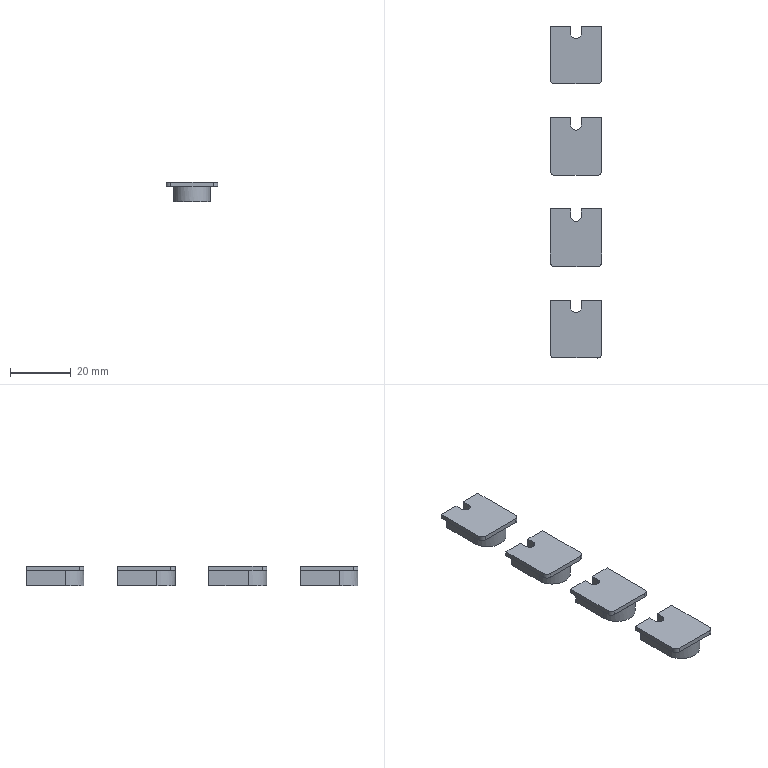CAM job | NX | 3-axis milling | part box 17.001 x 109 x 6.504 mm | stock box 20.002 x 114.001 x 10.005 mm
Tools:
number,name,description,diameter,corner_radius,flute_length,length,flutes
4,D4,平底铣刀-粗,4.0,0.0,25.0,75.0,2
9,D10,平底铣刀-粗,10.0,0.0,35.0,75.0,2
11,D3-J,平底铣刀-精,3.0,0.0,50.0,75.0,2
7,D6-J,平底铣刀-精,6.0,0.0,25.0,75.0,2
1,D80R0.8飞刀,圆鼻刀-粗,80.0,0.8,50.0,75.0,2
2,D6倒角刀,倒角刀,6.0,0.0,3.0,25.0,2
Operations:
program,operation,operation_type,tool,method,geometry_group,spindle_rpm,surface_speed,feed_per_tooth,feed_cut,feed_plunge,cut_length_mm,path_length_mm,cut_time_min,machine_time_min
A,顶面,FaceMilling,D80R0.8飞刀,侧刃精光-切深K-步距G,W-A,4000.0,1005.31,0.125,1000.0,100.0,203.0,239.0,0.203,0.2066
A,外形粗_2,VolumeBased25DMillingOperation,D10,METHOD,W-A,8000.0,251.327,0.3125,5000.0,80.0,4530.315,4862.015,0.9061,0.9392
A,底壁铣分层开粗-中_COPY,VolumeBased25DMillingOperation,D10,分层开粗-切深K-步距G,W-A,8000.0,251.32,0.25,4000.0,100.0,6989.181,8567.837,1.747,1.905
A,底壁粗_2,VolumeBased25DMillingOperation,D4,METHOD,W-A,6000.0,75.398,0.1,1200.0,100.0,1003.119,1717.466,0.8359,0.9074
A,底侧精_3,VolumeBased25DMillingOperation,D6-J,METHOD,W-A,6000.0,113.0,0.2083,1200.0,100.0,256.064,560.524,0.2134,0.2438
A,底侧精_4,VolumeBased25DMillingOperation,D6-J,METHOD,W-A,6000.0,113.0,0.2083,1200.0,100.0,64.508,338.62,0.0538,0.0812
A,外形侧面,ZLevelMilling,D3-J,METHOD,W-A,9000.0,84.823,0.1389,2500.0,80.0,574.358,860.838,0.2301,0.2587
A,仅选体,SurfaceContour,D6倒角刀,METHOD,W-A,8000.0,150.796,0.1875,3000.0,100.0,608.929,1372.217,0.203,0.2793
A,底壁铣倒角_COPY,VolumeBased25DMillingOperation,D6倒角刀,爬面_倒角-切深0-步距G,W-A,6500.0,122.519,0.1154,1500.0,100.0,101.228,347.592,0.0675,0.0921
A,外形半精_2,VolumeBased25DMillingOperation,D6-J,METHOD,W-A,8000.0,251.327,0.0625,1000.0,100.0,378.909,671.767,0.3789,0.4082